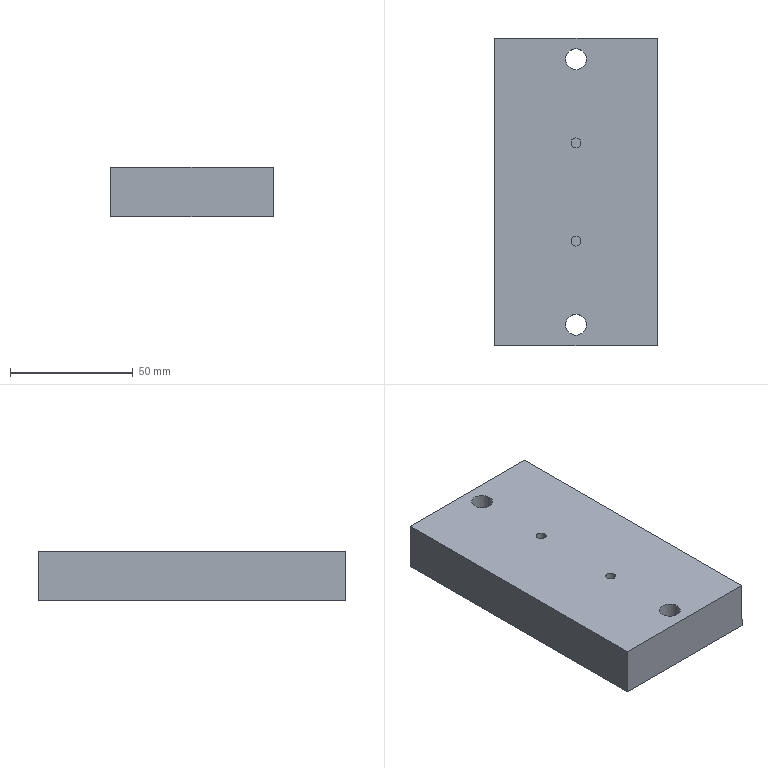NC program | NX | posted with a generic post | part box 65.936 x 125 x 20 mm
Lines 4573 to 6199 of 29196:
(FACE_MILLING_COPY , TOOL : D63)
N9024 T01 M6
N9026 G54
N9028 G17 G0 G90 X86.95 Y-24.269 S4000 M3
N9030 G43 Z37.5 H1
N9032 G94 G1 Z5.033 F5000.
N9034 X77.5 F2000.
N9036 X-77.5
N9038 Y24.269
N9040 X77.5
N9042 X86.95
N9044 G0 Z17.5
N9046 Y-24.269
N9048 G1 Z2.567 F5000.
N9050 X77.5 F2000.
N9052 X-77.5
N9054 Y24.269
N9056 X77.5
N9058 X86.95
N9060 G0 Z17.5
N9062 Y-24.269
N9064 G1 Z0.1 F5000.
N9066 X77.5 F2000.
N9068 X-77.5
N9070 Y24.269
N9072 X77.5
N9074 X86.95
N9076 G0 Z37.5
(FACE_MILLING_COPY_COPY , TOOL : D63)
N9078 Y-24.269
N9080 G1 Z0. F5000.
N9082 X77.5 F1000.
N9084 X-77.5
N9086 Y24.269
N9088 X77.5
N9090 X86.95
N9092 G0 Z37.5
(ZLEVEL_PROFILE_2 , TOOL : D63)
N9094 X86.434 Y-13.072
N9096 Z30.5
N9098 G1 Z-0.462 F5000.
N9100 X45.485 Y-13.396
N9102 X44.426 Y-13.405
N9104 X-45.488
N9106 X-86.438
N9108 G0 Y-15.399 Z-1.423
N9110 G1 X-45.488
N9112 X44.426
N9114 X45.485 Y-15.39
N9116 X86.434 Y-15.066
N9118 G0 Y-17.06 Z-2.385
N9120 G1 X45.485 Y-17.384
N9122 X44.426 Y-17.393
N9124 X-45.488
N9126 X-86.438
N9128 G0 Y-19.386 Z-3.347
N9130 G1 X-45.488
N9132 X44.426
N9134 X45.485 Y-19.378
N9136 X86.434 Y-19.054
N9138 G0 Y-21.048 Z-4.308
N9140 G1 X45.485 Y-21.372
N9142 X44.426 Y-21.38
N9144 X-45.488
N9146 X-86.438
N9148 G0 Y-23.374 Z-5.27
N9150 G1 X-45.488
N9152 X44.426
N9154 X45.485 Y-23.366
N9156 X86.434 Y-23.042
N9158 G0 Y-25.036 Z-6.232
N9160 G1 X45.485 Y-25.36
N9162 X44.426 Y-25.368
N9164 X-45.488
N9166 X-86.438
N9168 G0 Y-27.362 Z-7.193
N9170 G1 X-45.488
N9172 X44.426
N9174 X45.485 Y-27.354
N9176 X86.434 Y-27.029
N9178 G0 Y-29.023 Z-8.155
N9180 G1 X45.485 Y-29.347
N9182 X44.426 Y-29.356
N9184 X-45.488
N9186 X-86.438
N9188 G0 Y-31.35 Z-9.117
N9190 G1 X-45.488
N9192 X44.426
N9194 X45.485 Y-31.341
N9196 X86.434 Y-31.017
N9198 G0 Y-33.011 Z-10.078
N9200 G1 X45.485 Y-33.335
N9202 X44.426 Y-33.344
N9204 X-45.488
N9206 X-86.438
N9208 G0 Y-35.337 Z-11.04
N9210 G1 X-45.488
N9212 X44.426
N9214 X45.485 Y-35.329
N9216 X86.434 Y-35.005
N9218 G0 Y-36.999 Z-12.001
N9220 G1 X45.485 Y-37.323
N9222 X44.426 Y-37.331
N9224 X-45.488
N9226 X-86.438
N9228 G0 Y-39.325 Z-12.963
N9230 G1 X-45.488
N9232 X45.536
N9234 X86.486
N9236 G0 Z30.5
(ZLEVEL_PROFILE_2_COPY , TOOL : D63)
N9238 X-86.435 Y52.145
N9240 G1 Z-0.479
N9242 X-45.485 Y52.148
N9244 X-45.372
N9246 X44.666
N9248 X45.485 Y52.144
N9250 X86.435 Y51.946
N9252 G0 X86.434 Y52.458 Z-1.457
N9254 G1 X45.485 Y52.832
N9256 X45.372 Y52.833
N9258 X-45.372
N9260 X-45.485 Y52.832
N9262 X-86.434 Y52.458
N9264 G0 X-86.435 Y53.316 Z-2.436
N9266 G1 X-45.485 Y53.514
N9268 X-44.666 Y53.518
N9270 X44.666
N9272 X45.485 Y53.514
N9274 X86.435 Y53.316
N9276 G0 X86.434 Y53.829 Z-3.414
N9278 G1 X45.485 Y54.202
N9280 X45.372 Y54.203
N9282 X-45.372
N9284 X-45.485 Y54.202
N9286 X-86.434 Y53.829
N9288 G0 X-86.435 Y54.887 Z-4.393
N9290 G1 X-45.485 Y54.889
N9292 X-45.484
N9294 X44.666
N9296 X45.485 Y54.885
N9298 X86.435 Y54.686
N9300 G0 Y55.372 Z-5.371
N9302 G1 X45.485 Y55.57
N9304 X44.666 Y55.574
N9306 X-44.666
N9308 X-45.485 Y55.57
N9310 X-86.435 Y55.372
N9312 G0 Y56.057 Z-6.35
N9314 G1 X-45.485 Y56.255
N9316 X-44.666 Y56.259
N9318 X44.666
N9320 X45.485 Y56.255
N9322 X86.435 Y56.057
N9324 G0 Y56.742 Z-7.329
N9326 G1 X45.485 Y56.94
N9328 X44.666 Y56.944
N9330 X-44.666
N9332 X-45.485 Y56.94
N9334 X-86.435 Y56.742
N9336 G0 X-86.434 Y57.255 Z-8.307
N9338 G1 X-45.485 Y57.628
N9340 X-45.372 Y57.629
N9342 X45.372
N9344 X45.485 Y57.628
N9346 X86.434 Y57.255
N9348 G0 X86.435 Y58.113 Z-9.286
N9350 G1 X45.485 Y58.311
N9352 X44.666 Y58.315
N9354 X-45.372
N9356 X-45.485 Y58.314
N9358 X-86.434 Y57.94
N9360 G0 Y58.625 Z-10.264
N9362 G1 X-45.485 Y58.999
N9364 X-45.372 Y59.
N9366 X45.372
N9368 X45.485 Y58.999
N9370 X86.434 Y58.625
N9372 G0 X86.435 Y59.483 Z-11.243
N9374 G1 X45.485 Y59.681
N9376 X44.666 Y59.685
N9378 X-44.666
N9380 X-45.485 Y59.681
N9382 X-86.435 Y59.483
N9384 G0 Y60.369 Z-12.221
N9386 G1 X-45.485 Y60.37
N9388 X-45.372
N9390 X44.666
N9392 X45.485 Y60.366
N9394 X86.435 Y60.168
N9396 G0 Y61.055 Z-13.2
N9398 G1 X45.485
N9400 X-45.
N9402 X-45.449 Y61.053
N9404 X-86.398 Y60.798
N9406 G0 Z30.5
(ZLEVEL_PROFILE_2_COPY_COPY , TOOL : D63)
N9408 X-86.435 Y66.087
N9410 Z16.974
N9412 G1 Z-14.388
N9414 X-45.485 Y66.088 F4500.
N9416 X-45.372 Y66.087
N9418 X45.372
N9420 X45.485 Y66.088
N9422 X86.435 Y66.087
N9424 G0 X86.436 Y66.761 Z-15.351
N9426 G1 X45.486 Y66.762
N9428 X45.372
N9430 X-45.372
N9432 X-45.486
N9434 X-86.436 Y66.761
N9436 G0 Y67.435 Z-16.315
N9438 G1 X-45.486 Y67.437
N9440 X-45.372 Y67.436
N9442 X45.372
N9444 X45.486 Y67.437
N9446 X86.436 Y67.435
N9448 G0 Y68.11 Z-17.278
N9450 G1 X45.486 Y68.111
N9452 X45.372
N9454 X-45.372
N9456 X-45.486
N9458 X-86.436 Y68.11
N9460 G0 Y68.784 Z-18.241
N9462 G1 X-45.486 Y68.785
N9464 X-45.485
N9466 X45.485
N9468 X45.486
N9470 X86.436 Y68.784
N9472 G0 Y69.46 Z-19.204
N9474 G1 X45.486
N9476 X-45.486
N9478 X-86.436
N9480 G0 Y70.134 Z-20.168
N9482 G1 X-45.486
N9484 X45.486
N9486 X86.436
N9488 G0 Y70.809 Z-21.131
N9490 G1 X45.486
N9492 X-45.486
N9494 X-86.436
N9496 G0 Y71.483 Z-22.094
N9498 G1 X-45.486 Y71.484
N9500 X-45.372 Y71.483
N9502 X45.372
N9504 X45.486 Y71.484
N9506 X86.436 Y71.483
N9508 G0 Y72.158 Z-23.058
N9510 G1 X45.486
N9512 X45.372
N9514 X-45.372
N9516 X-45.486
N9518 X-86.436
N9520 G0 X-86.435 Y72.832 Z-24.021
N9522 G1 X-45.485 Y72.833
N9524 X-45.372 Y72.832
N9526 X45.372
N9528 X45.485 Y72.833
N9530 X86.435 Y72.832
N9532 G0 Y73.507 Z-24.984
N9534 G1 X45.485
N9536 X-45.485
N9538 X-86.435
N9540 G0 Z16.974
(PLANAR_MILL_1_COPY_COPY_COPY_COPY_1 , TOOL : D63)
N9542 X83.8 Y-66.
N9544 Z9.801
N9546 G1 Y-58.235 Z-19.177 F5000.
N9548 X46. F1200.
N9550 X-46.
N9552 X-83.8
N9554 G0 Y-66. Z9.801
N9556 M5
(PLANAR_MILL_1_COPY_COPY_COPY , TOOL : D6R0)
N9558 T09 M6
N9560 G54
N9562 G17 G0 G90 X-27.791 Y-24.135 S8000 M3
N9564 G43 Z17.075 H9
N9566 G94 G1 Z-12.325 F5000.
N9568 X-39.095 Z-12.404 F2000.
N9570 X-39.333 Y-24.194 Z-12.405
N9572 X-39.547 Y-24.314 Z-12.407
N9574 X-39.721 Y-24.488 Z-12.409
N9576 X-39.841 Y-24.702 Z-12.411
N9578 X-39.9 Y-24.94 Z-12.412
N9580 Y-28.13 Z-12.435
N9582 X-39.841 Y-28.369 Z-12.436
N9584 X-39.721 Y-28.582 Z-12.438
N9586 X-39.547 Y-28.756 Z-12.44
N9588 X-39.333 Y-28.877 Z-12.441
N9590 X-39.095 Y-28.935 Z-12.443
N9592 X39.095 Z-12.989
N9594 X39.333 Y-28.877 Z-12.991
N9596 X39.547 Y-28.756 Z-12.992
N9598 X39.721 Y-28.582 Z-12.994
N9600 X39.841 Y-28.369 Z-12.996
N9602 X39.9 Y-28.13 Z-12.998
N9604 Y-24.94 Z-13.02
N9606 X39.841 Y-24.702 Z-13.022
N9608 X39.721 Y-24.488 Z-13.023
N9610 X39.547 Y-24.314 Z-13.025
N9612 X39.333 Y-24.194 Z-13.027
N9614 X39.095 Y-24.135 Z-13.028
N9616 X-39.095 Z-13.574
N9618 X-39.333 Y-24.194 Z-13.576
N9620 X-39.547 Y-24.314 Z-13.578
N9622 X-39.721 Y-24.488 Z-13.579
N9624 X-39.841 Y-24.702 Z-13.581
N9626 X-39.9 Y-24.94 Z-13.583
N9628 Y-28.13 Z-13.605
N9630 X-39.841 Y-28.369 Z-13.607
N9632 X-39.721 Y-28.582 Z-13.609
N9634 X-39.547 Y-28.756 Z-13.61
N9636 X-39.333 Y-28.877 Z-13.612
N9638 X-39.095 Y-28.935 Z-13.614
N9640 X39.095 Z-14.16
N9642 X39.333 Y-28.877 Z-14.161
N9644 X39.547 Y-28.756 Z-14.163
N9646 X39.721 Y-28.582 Z-14.165
N9648 X39.841 Y-28.369 Z-14.166
N9650 X39.9 Y-28.13 Z-14.168
N9652 Y-24.94 Z-14.19
N9654 X39.841 Y-24.702 Z-14.192
N9656 X39.721 Y-24.488 Z-14.194
N9658 X39.547 Y-24.314 Z-14.196
N9660 X39.333 Y-24.194 Z-14.197
N9662 X39.095 Y-24.135 Z-14.199
N9664 X-39.095 Z-14.745
N9666 X-39.333 Y-24.194 Z-14.747
N9668 X-39.547 Y-24.314 Z-14.748
N9670 X-39.721 Y-24.488 Z-14.75
N9672 X-39.841 Y-24.702 Z-14.752
N9674 X-39.9 Y-24.94 Z-14.753
N9676 Y-28.13 Z-14.776
N9678 X-39.841 Y-28.369 Z-14.777
N9680 X-39.721 Y-28.582 Z-14.779
N9682 X-39.547 Y-28.756 Z-14.781
N9684 X-39.333 Y-28.877 Z-14.783
N9686 X-39.095 Y-28.935 Z-14.784
N9688 X39.095 Z-15.33
N9690 X39.333 Y-28.877 Z-15.332
N9692 X39.547 Y-28.756 Z-15.334
N9694 X39.721 Y-28.582 Z-15.335
N9696 X39.841 Y-28.369 Z-15.337
N9698 X39.9 Y-28.13 Z-15.339
N9700 Y-24.94 Z-15.361
N9702 X39.841 Y-24.702 Z-15.363
N9704 X39.721 Y-24.488 Z-15.364
N9706 X39.547 Y-24.314 Z-15.366
N9708 X39.333 Y-24.194 Z-15.368
N9710 X39.095 Y-24.135 Z-15.37
N9712 X-39.095 Z-15.915
N9714 X-39.333 Y-24.194 Z-15.917
N9716 X-39.547 Y-24.314 Z-15.919
N9718 X-39.721 Y-24.488 Z-15.921
N9720 X-39.841 Y-24.702 Z-15.922
N9722 X-39.9 Y-24.94 Z-15.924
N9724 Y-28.13 Z-15.946
N9726 X-39.841 Y-28.369 Z-15.948
N9728 X-39.721 Y-28.582 Z-15.95
N9730 X-39.547 Y-28.756 Z-15.951
N9732 X-39.333 Y-28.877 Z-15.953
N9734 X-39.095 Y-28.935 Z-15.955
N9736 X39.095 Z-16.501
N9738 X39.333 Y-28.877 Z-16.502
N9740 X39.547 Y-28.756 Z-16.504
N9742 X39.721 Y-28.582 Z-16.506
N9744 X39.841 Y-28.369 Z-16.508
N9746 X39.9 Y-28.13 Z-16.509
N9748 Y-24.94 Z-16.532
N9750 X39.841 Y-24.702 Z-16.533
N9752 X39.721 Y-24.488 Z-16.535
N9754 X39.547 Y-24.314 Z-16.537
N9756 X39.333 Y-24.194 Z-16.538
N9758 X39.095 Y-24.135 Z-16.54
N9760 X-39.095 Z-17.086
N9762 X-39.333 Y-24.194 Z-17.088
N9764 X-39.547 Y-24.314 Z-17.089
N9766 X-39.721 Y-24.488 Z-17.091
N9768 X-39.841 Y-24.702 Z-17.093
N9770 X-39.9 Y-24.94 Z-17.095
N9772 Y-28.13 Z-17.117
N9774 X-39.841 Y-28.369 Z-17.119
N9776 X-39.721 Y-28.582 Z-17.12
N9778 X-39.547 Y-28.756 Z-17.122
N9780 X-39.333 Y-28.877 Z-17.124
N9782 X-39.095 Y-28.935 Z-17.125
N9784 X39.095 Z-17.671
N9786 X39.333 Y-28.877 Z-17.673
N9788 X39.547 Y-28.756 Z-17.675
N9790 X39.721 Y-28.582 Z-17.676
N9792 X39.841 Y-28.369 Z-17.678
N9794 X39.9 Y-28.13 Z-17.68
N9796 Y-24.94 Z-17.702
N9798 X39.841 Y-24.702 Z-17.704
N9800 X39.721 Y-24.488 Z-17.706
N9802 X39.547 Y-24.314 Z-17.707
N9804 X39.333 Y-24.194 Z-17.709
N9806 X39.095 Y-24.135 Z-17.711
N9808 X-39.095 Z-18.257
N9810 X-39.333 Y-24.194 Z-18.258
N9812 X-39.547 Y-24.314 Z-18.26
N9814 X-39.721 Y-24.488 Z-18.262
N9816 X-39.841 Y-24.702 Z-18.263
N9818 X-39.9 Y-24.94 Z-18.265
N9820 Y-28.13 Z-18.287
N9822 X-39.841 Y-28.369 Z-18.289
N9824 X-39.721 Y-28.582 Z-18.291
N9826 X-39.547 Y-28.756 Z-18.293
N9828 X-39.333 Y-28.877 Z-18.294
N9830 X-39.095 Y-28.935 Z-18.296
N9832 X39.095 Z-18.842
N9834 X39.333 Y-28.877 Z-18.844
N9836 X39.547 Y-28.756 Z-18.845
N9838 X39.721 Y-28.582 Z-18.847
N9840 X39.841 Y-28.369 Z-18.849
N9842 X39.9 Y-28.13 Z-18.85
N9844 Y-24.94 Z-18.873
N9846 X39.841 Y-24.702 Z-18.874
N9848 X39.721 Y-24.488 Z-18.876
N9850 X39.547 Y-24.314 Z-18.878
N9852 X39.333 Y-24.194 Z-18.88
N9854 X39.095 Y-24.135 Z-18.881
N9856 X-39.095 Z-19.427
N9858 X-39.333 Y-24.194 Z-19.429
N9860 X-39.547 Y-24.314 Z-19.431
N9862 X-39.721 Y-24.488 Z-19.432
N9864 X-39.841 Y-24.702 Z-19.434
N9866 X-39.9 Y-24.94 Z-19.436
N9868 Y-28.13 Z-19.458
N9870 X-39.841 Y-28.369 Z-19.46
N9872 X-39.721 Y-28.582 Z-19.461
N9874 X-39.547 Y-28.756 Z-19.463
N9876 X-39.333 Y-28.877 Z-19.465
N9878 X-39.095 Y-28.935 Z-19.467
N9880 X39.095 Z-20.012
N9882 X39.333 Y-28.877 Z-20.014
N9884 X39.547 Y-28.756 Z-20.016
N9886 X39.721 Y-28.582 Z-20.018
N9888 X39.841 Y-28.369 Z-20.019
N9890 X39.9 Y-28.13 Z-20.021
N9892 Y-24.94 Z-20.043
N9894 X39.841 Y-24.702 Z-20.045
N9896 X39.721 Y-24.488 Z-20.047
N9898 X39.547 Y-24.314 Z-20.048
N9900 X39.333 Y-24.194 Z-20.05
N9902 X39.095 Y-24.135 Z-20.052
N9904 X0. Z-20.325
N9906 X-39.
N9908 G3 X-39.9 Y-25.035 R0.9
N9910 G1 Y-28.035
N9912 G3 X-39. Y-28.935 R0.9
N9914 G1 X39.
N9916 G3 X39.9 Y-28.035 R0.9
N9918 G1 Y-25.035
N9920 G3 X39. Y-24.135 R0.9
N9922 G1 X0.
N9924 G0 Z17.075
(PLANAR_MILL_1_COPY_COPY_COPY_COPY , TOOL : D6R0)
N9926 X0.75 Y-25.468
N9928 G1 Z-20.275 F5000.
N9930 Z-20.425 F100.
N9932 G41 X1. Y-25.035 D9
N9934 G3 X0. Y-24.035 R1.
N9936 G1 X-39. F800.
N9938 G3 X-40. Y-25.035 R1.
N9940 G1 Y-28.035
N9942 G3 X-39. Y-29.035 R1.
N9944 G1 X39.
N9946 G3 X40. Y-28.035 R1.
N9948 G1 Y-25.035
N9950 G3 X39. Y-24.035 R1.
N9952 G1 X0.
N9954 X-0.3
N9956 G3 X-1.3 Y-25.035 R1.
N9958 G40
N9960 G1 X-1.05 Y-25.468
N9962 Z-20.275
N9964 G0 Z17.075
(CAVITY_MILL , TOOL : D6R0)
N9966 Z30.
N9968 X49.62 Y-37.802
N9970 G1 Z-13.916 F5000.
N9972 X46.02 F4500.
N9974 Y-39.046
N9976 Y-39.219
N9978 Y-41.432
N9980 X46.014 Y-41.446
N9982 X45.8 Y-41.654
N9984 X43.014 Y-44.346
N9986 X43. Y-44.352
N9988 X38.561 Y-44.35
N9990 X38.536 Y-44.346
N9992 X38.533 Y-44.318
N9994 X38.557 Y-44.31
N9996 X38.604 Y-44.3
N9998 X38.723 Y-44.275
N10000 X38.826 Y-44.248
N10002 X38.929 Y-44.218
N10004 X39.066 Y-44.171
N10006 X39.363 Y-44.043
N10008 X39.41 Y-44.019
N10010 X39.754 Y-43.813
N10012 X39.907 Y-43.7
N10014 X40.097 Y-43.536
N10016 X40.276 Y-43.356
N10018 X40.441 Y-43.16
N10020 X40.547 Y-43.012
N10022 X40.75 Y-42.668
N10024 X40.784 Y-42.598
N10026 X40.898 Y-42.325
N10028 X41. Y-41.981
N10030 X41.059 Y-41.638
N10032 X41.08 Y-41.293
N10034 Y-40.953
N10036 Y-40.948
N10038 Y-40.256
N10040 Y-39.144
N10042 X41.2
N10044 G3 X44.3 Y-36.044 R3.1
N10046 G1 Y-35.499
N10048 G3 X46.01 Y-34.155 R3.1
N10050 G1 X46.026 Y-34.157
N10052 X46.02 Y-34.172
N10054 Y-37.802
N10056 X49.62
N10058 G0 Z-13.125
N10060 G1 Z-14.407 F5000.
N10062 X46.02 F4500.
N10064 Y-39.046
N10066 Y-39.219
N10068 Y-41.432
N10070 X46.014 Y-41.446
N10072 X45.8 Y-41.654
N10074 X43.014 Y-44.346
N10076 X43. Y-44.352
N10078 X38.561 Y-44.35
N10080 X38.536 Y-44.346
N10082 X38.533 Y-44.318
N10084 X38.557 Y-44.31
N10086 X38.604 Y-44.3
N10088 X38.723 Y-44.275
N10090 X38.826 Y-44.248
N10092 X38.929 Y-44.218
N10094 X39.066 Y-44.171
N10096 X39.363 Y-44.043
N10098 X39.41 Y-44.019
N10100 X39.754 Y-43.813
N10102 X39.907 Y-43.7
N10104 X40.097 Y-43.536
N10106 X40.276 Y-43.356
N10108 X40.441 Y-43.16
N10110 X40.547 Y-43.012
N10112 X40.75 Y-42.668
N10114 X40.784 Y-42.598
N10116 X40.898 Y-42.325
N10118 X41. Y-41.981
N10120 X41.059 Y-41.638
N10122 X41.08 Y-41.293
N10124 Y-40.953
N10126 Y-40.948
N10128 Y-40.795
N10130 G3 X41.1 Y-40.433 R5.336
N10132 G1 Y-39.144
N10134 X41.2
N10136 G3 X44.3 Y-36.044 R3.1
N10138 G1 Y-35.499
N10140 G3 X46.01 Y-34.155 R3.1
N10142 G1 X46.026 Y-34.157
N10144 X46.02 Y-34.172
N10146 Y-37.802
N10148 X49.62
N10150 G0 Z-13.616
N10152 G1 Z-14.898 F5000.
N10154 X46.02 F4500.
N10156 Y-39.046
N10158 Y-39.219
N10160 Y-41.432
N10162 X46.014 Y-41.446
N10164 X45.8 Y-41.654
N10166 X43.014 Y-44.346
N10168 X43. Y-44.352
N10170 X38.561 Y-44.35
N10172 X38.541 Y-44.352
N10174 Y-44.332
N10176 G3 X41.1 Y-41.21 R3.106
N10178 G1 Y-39.144
N10180 X41.2
N10182 G3 X44.3 Y-36.044 R3.1
N10184 G1 Y-35.499
N10186 G3 X46.01 Y-34.155 R3.1
N10188 G1 X46.026 Y-34.157
N10190 X46.02 Y-34.172
N10192 Y-37.802
N10194 X49.62
N10196 G0 Z-14.107
N10198 G1 Z-15.388 F5000.
N10200 X46.02 F4500.
N10202 Y-39.046
N10204 Y-39.219
N10206 Y-41.432
N10208 X46.014 Y-41.446
N10210 X45.8 Y-41.654
N10212 X43.014 Y-44.346
N10214 X43. Y-44.352
N10216 X38.561 Y-44.35
N10218 X38.541 Y-44.352
N10220 Y-44.332
N10222 G3 X41.1 Y-41.078 R3.12
N10224 G1 Y-39.144
N10226 X41.2
N10228 G3 X44.3 Y-36.044 R3.1
N10230 G1 Y-35.499
N10232 G3 X46.01 Y-34.155 R3.1
N10234 G1 X46.026 Y-34.157
N10236 X46.02 Y-34.172
N10238 Y-37.802
N10240 X49.62
N10242 G0 Z-14.598
N10244 G1 Z-15.879 F5000.
N10246 X46.02 F4500.
N10248 Y-39.046
N10250 Y-39.219
N10252 Y-41.432
N10254 X46.014 Y-41.446
N10256 X45.8 Y-41.654
N10258 X43.014 Y-44.346
N10260 X43. Y-44.352
N10262 X38.561 Y-44.35
N10264 X38.542 Y-44.353
N10266 Y-44.333
N10268 G3 X41.1 Y-41.252 R3.103
N10270 G1 Y-39.144
N10272 X41.2
N10274 G3 X44.3 Y-36.044 R3.1
N10276 G1 Y-35.499
N10278 G3 X46.01 Y-34.155 R3.1
N10280 G1 X46.026 Y-34.157
N10282 X46.02 Y-34.172
N10284 Y-37.802
N10286 X49.62
N10288 G0 Z-15.088
N10290 G1 Z-16.37 F5000.
N10292 X46.02 F4500.
N10294 Y-39.046
N10296 Y-39.219
N10298 Y-41.432
N10300 X46.014 Y-41.446
N10302 X45.8 Y-41.654
N10304 X43.014 Y-44.346
N10306 X43. Y-44.352
N10308 X38.561 Y-44.35
N10310 X38.542 Y-44.353
N10312 X38.541 Y-44.333
N10314 G3 X41.1 Y-41.259 R3.102
N10316 G1 Y-39.144
N10318 X41.2
N10320 G3 X44.3 Y-36.044 R3.1
N10322 G1 Y-35.499
N10324 G3 X46.01 Y-34.155 R3.1
N10326 G1 X46.026 Y-34.157
N10328 X46.02 Y-34.172
N10330 Y-37.802
N10332 X49.62
N10334 G0 Z-15.579
N10336 G1 Z-16.861 F5000.
N10338 X46.02 F4500.
N10340 Y-39.046
N10342 Y-39.219
N10344 Y-41.432
N10346 X46.014 Y-41.446
N10348 X45.8 Y-41.654
N10350 X43.014 Y-44.346
N10352 X43. Y-44.352
N10354 X38.561 Y-44.35
N10356 X38.542 Y-44.353
N10358 X38.541 Y-44.333
N10360 G3 X41.1 Y-41.267 R3.102
N10362 G1 Y-39.144
N10364 X41.2
N10366 G3 X44.3 Y-36.044 R3.1
N10368 G1 Y-35.499
N10370 G3 X46.01 Y-34.155 R3.1
N10372 G1 X46.026 Y-34.157
N10374 X46.02 Y-34.172
N10376 Y-37.802
N10378 X49.62
N10380 G0 Z-16.07
N10382 G1 Z-17.352 F5000.
N10384 X46.02 F4500.
N10386 Y-39.046
N10388 Y-39.219
N10390 Y-41.432
N10392 X46.014 Y-41.446
N10394 X45.8 Y-41.654
N10396 X43.014 Y-44.346
N10398 X43. Y-44.352
N10400 X38.561 Y-44.35
N10402 X38.542 Y-44.353
N10404 X38.541 Y-44.333
N10406 G3 X41.1 Y-41.274 R3.101
N10408 G1 Y-39.144
N10410 X41.2
N10412 G3 X44.3 Y-36.044 R3.1
N10414 G1 Y-35.499
N10416 G3 X46.01 Y-34.155 R3.1
N10418 G1 X46.026 Y-34.157
N10420 X46.02 Y-34.172
N10422 Y-37.802
N10424 X49.62
N10426 G0 Z-16.561
N10428 G1 Z-17.843 F5000.
N10430 X46.02 F4500.
N10432 Y-39.046
N10434 Y-39.219
N10436 Y-41.432
N10438 X46.014 Y-41.446
N10440 X45.8 Y-41.654
N10442 X43.014 Y-44.346
N10444 X43. Y-44.352
N10446 X38.561 Y-44.35
N10448 X38.541 Y-44.352
N10450 Y-44.332
N10452 G3 X41.1 Y-41.282 R3.107
N10454 G1 Y-39.144
N10456 X41.2
N10458 G3 X44.3 Y-36.044 R3.1
N10460 G1 Y-35.499
N10462 G3 X46.01 Y-34.155 R3.1
N10464 G1 X46.026 Y-34.157
N10466 X46.02 Y-34.172
N10468 Y-37.802
N10470 X49.62
N10472 G0 Z-17.052
N10474 G1 Z-18.334 F5000.
N10476 X46.02 F4500.
N10478 Y-39.046
N10480 Y-39.219
N10482 Y-41.432
N10484 X46.014 Y-41.446
N10486 X45.8 Y-41.654
N10488 X43.014 Y-44.346
N10490 X43. Y-44.352
N10492 X38.561 Y-44.35
N10494 X38.542 Y-44.353
N10496 Y-44.334
N10498 G3 X41.1 Y-41.289 R3.096
N10500 G1 Y-39.144
N10502 X41.2
N10504 G3 X44.3 Y-36.044 R3.1
N10506 G1 Y-35.499
N10508 G3 X46.01 Y-34.155 R3.1
N10510 G1 X46.026 Y-34.157
N10512 X46.02 Y-34.172
N10514 Y-37.802
N10516 X49.62
N10518 G0 Z-17.543
N10520 G1 Z-18.825 F5000.
N10522 X46.02 F4500.
N10524 Y-39.046
N10526 Y-39.219
N10528 Y-41.432
N10530 X46.014 Y-41.446
N10532 X45.8 Y-41.654
N10534 X43.014 Y-44.346
N10536 X43. Y-44.352
N10538 X38.561 Y-44.35
N10540 X38.543 Y-44.354
N10542 X38.542 Y-44.335
N10544 G3 X41.049 Y-41.827 R3.079
N10546 X41.1 Y-40.948 R3.891
N10548 G1 Y-39.144
N10550 X41.2
N10552 G3 X44.3 Y-36.044 R3.1
N10554 G1 Y-35.499
N10556 G3 X46.01 Y-34.155 R3.1
N10558 G1 X46.026 Y-34.157
N10560 X46.02 Y-34.172
N10562 Y-37.802
N10564 X49.62
N10566 G0 Z-18.034
N10568 X47.015 Y-45.486
N10570 G1 Z-19.202 F5000.
N10572 X44.514 Y-42.897 F4500.
N10574 X43.014 Y-44.346
N10576 X43. Y-44.352
N10578 X38.561 Y-44.35
N10580 X38.542 Y-44.353
N10582 X38.541 Y-44.333
N10584 G3 X41.029 Y-41.939 R3.1
N10586 X41.1 Y-40.948 R4.04
N10588 G1 Y-40.466
N10590 X46.
N10592 X46.02
N10594 Y-41.432
N10596 X46.014 Y-41.446
N10598 X45.8 Y-41.654
N10600 X44.514 Y-42.897
N10602 X47.015 Y-45.486
N10604 G0 Z-18.525
N10606 G1 Z-19.58 F5000.
N10608 X44.514 Y-42.897 F4500.
N10610 X43.014 Y-44.346
N10612 X43. Y-44.352
N10614 X38.561 Y-44.35
N10616 X38.541 Y-44.352
N10618 Y-44.332
N10620 G3 X41.043 Y-41.875 R3.097
N10622 G1 X45.544
N10624 X45.572
N10626 X45.562 Y-41.884
N10628 X44.514 Y-42.897
N10630 X47.015 Y-45.486
N10632 G0 Z-18.902
N10634 X40.779 Y-47.951
N10636 G1 Z-19.957 F5000.
N10638 X40.78 Y-44.351 F4500.
N10640 X38.561 Y-44.35
N10642 X38.542 Y-44.353
N10644 X38.541 Y-44.333
N10646 G3 X40.366 Y-43.284 R3.103
N10648 G1 X44.085
N10650 X44.115 Y-43.282
N10652 X44.104 Y-43.293
N10654 X43.014 Y-44.346
N10656 X43. Y-44.352
N10658 X40.78 Y-44.351
N10660 X40.779 Y-47.951
N10662 G0 Z30.
N10664 X0. Y-28.415
N10666 G1 Z-13.916 F5000.
N10668 Y-32.015 F4500.
N10670 X35.9
N10672 Y-32.035
N10674 Y-35.789
N10676 X35.616
N10678 X-35.9
N10680 Y-32.035
N10682 Y-32.015
N10684 X0.
N10686 Y-28.415
N10688 G0 Z-13.125
N10690 G1 Z-14.407 F5000.
N10692 Y-32.015 F4500.
N10694 X35.9
N10696 Y-32.035
N10698 Y-35.65
N10700 X-35.9
N10702 Y-32.035
N10704 Y-32.015
N10706 X0.
N10708 Y-28.415
N10710 G0 Z-13.616
N10712 G1 Z-14.898 F5000.
N10714 Y-32.015 F4500.
N10716 X35.9
N10718 Y-32.035
N10720 Y-35.518
N10722 X-35.9
N10724 Y-32.035
N10726 Y-32.015
N10728 X0.
N10730 Y-28.415
N10732 G0 Z-14.107
N10734 G1 Z-15.388 F5000.
N10736 Y-32.015 F4500.
N10738 X35.9
N10740 Y-32.035
N10742 Y-35.387
N10744 X-35.9
N10746 Y-32.035
N10748 Y-32.015
N10750 X0.
N10752 Y-28.415
N10754 G0 Z-14.598
N10756 G1 Z-15.879 F5000.
N10758 Y-32.015 F4500.
N10760 X35.9
N10762 Y-32.035
N10764 Y-35.255
N10766 X35.61
N10768 X35.27 Y-35.274
N10770 G2 X34.859 Y-35.289 R1.231
N10772 G3 X34.39 Y-35.255 R3.884
N10774 G1 X0.61
N10776 G3 X0. Y-35.313 R3.285
N10778 X-0.61 Y-35.255 R3.616
N10780 G1 X-34.39
N10782 G3 X-34.862 Y-35.289 R3.884
N10784 G2 X-35.27 Y-35.273 R1.193
N10786 G1 X-35.61 Y-35.255
N10788 X-35.9
N10790 Y-32.035
N10792 Y-32.015
N10794 X0.
N10796 Y-28.415
N10798 G0 Z-15.088
N10800 G1 Z-16.37 F5000.
N10802 Y-32.015 F4500.
N10804 X35.9
N10806 Y-32.035
N10808 Y-35.124
N10810 X35.8
N10812 G3 X34.998 Y-35.226 R2.948
N10814 X34.231 Y-35.124 R3.08
N10816 G1 X34.2
N10818 X0.8
N10820 G3 X0. Y-35.226 R3.067
N10822 X-0.8 Y-35.124 R3.164
N10824 G1 X-34.2
N10826 G3 X-35.002 Y-35.227 R3.207
N10828 X-35.8 Y-35.124 R2.985
N10830 G1 X-35.9
N10832 Y-32.035
N10834 Y-32.015
N10836 X0.
N10838 Y-28.415
N10840 G0 Z-15.579
N10842 G1 Z-16.861 F5000.
N10844 Y-32.015 F4500.
N10846 X35.9
N10848 Y-32.035
N10850 Y-34.992
N10852 X35.618
N10854 G3 X35.169 Y-35.024 R3.541
N10856 G2 X34.578 Y-34.999 R1.703
N10858 G1 X34.382 Y-34.992
N10860 X0.618
N10862 G3 X0. Y-35.052 R3.363
N10864 X-0.618 Y-34.992 R3.433
N10866 G1 X-34.382
N10868 G3 X-34.853 Y-35.028 R3.234
N10870 G2 X-35.27 Y-35.011 R1.114
N10872 G1 X-35.618 Y-34.992
N10874 X-35.9
N10876 Y-32.035
N10878 Y-32.015
N10880 X0.
N10882 Y-28.415
N10884 G0 Z-16.07
N10886 G1 Z-17.352 F5000.
N10888 Y-32.015 F4500.
N10890 X35.9
N10892 Y-32.035
N10894 Y-34.861
N10896 X-35.9
N10898 Y-32.035
N10900 Y-32.015
N10902 X0.
N10904 Y-28.415
N10906 G0 Z-16.561
N10908 G1 Z-17.843 F5000.
N10910 Y-32.015 F4500.
N10912 X35.9
N10914 Y-32.035
N10916 Y-34.729
N10918 X-35.9
N10920 Y-32.035
N10922 Y-32.015
N10924 X0.
N10926 Y-28.415
N10928 G0 Z-17.052
N10930 G1 Z-18.334 F5000.
N10932 Y-32.015 F4500.
N10934 X35.9
N10936 Y-32.035
N10938 Y-34.598
N10940 X-35.9
N10942 Y-32.035
N10944 Y-32.015
N10946 X0.
N10948 Y-28.415
N10950 G0 Z-17.543
N10952 G1 Z-18.825 F5000.
N10954 Y-32.015 F4500.
N10956 X35.9
N10958 Y-32.035
N10960 Y-34.467
N10962 X-35.9
N10964 Y-32.035
N10966 Y-32.015
N10968 X0.
N10970 Y-28.415
N10972 G0 Z30.
N10974 X-49.62 Y-37.806
N10976 G1 Z-13.916 F5000.
N10978 X-46.02 F4500.
N10980 Y-34.376
N10982 Y-34.375
N10984 X-46.01 Y-34.181
N10986 X-46.003 Y-34.167
N10988 G3 X-44.3 Y-35.499 R3.1
N10990 G1 Y-36.044
N10992 G3 X-41.2 Y-39.144 R3.1
N10994 G1 X-41.08
N10996 X-41.07 Y-40.256
N10998 Y-40.433
N11000 Y-40.948
N11002 Y-41.294
N11004 X-41.059 Y-41.638
N11006 X-41. Y-41.981
N11008 X-40.898 Y-42.325
N11010 X-40.784 Y-42.598
N11012 X-40.75 Y-42.668
N11014 X-40.547 Y-43.012
N11016 X-40.441 Y-43.16
N11018 X-40.276 Y-43.356
N11020 X-40.097 Y-43.536
N11022 X-39.907 Y-43.7
N11024 X-39.754 Y-43.813
N11026 X-39.41 Y-44.019
N11028 X-39.363 Y-44.043
N11030 X-39.066 Y-44.171
N11032 X-38.929 Y-44.218
N11034 X-38.826 Y-44.248
N11036 X-38.723 Y-44.275
N11038 X-38.547 Y-44.312
N11040 X-38.523 Y-44.321
N11042 X-38.526 Y-44.349
N11044 X-38.551 Y-44.352
N11046 X-42.956
N11048 X-42.968 Y-44.347
N11050 X-42.995 Y-44.326
N11052 X-43.235 Y-44.13
N11054 X-43.237 Y-44.129
N11056 X-45.442 Y-42.
N11058 X-46.014 Y-41.446
N11060 X-46.02 Y-41.432
N11062 Y-39.219
N11064 Y-39.046
N11066 Y-37.806
N11068 X-49.62
N11070 G0 Z-13.125
N11072 G1 Z-14.407 F5000.
N11074 X-46.02 F4500.
N11076 Y-34.376
N11078 Y-34.375
N11080 X-46.01 Y-34.181
N11082 X-46.003 Y-34.167
N11084 G3 X-44.3 Y-35.499 R3.1
N11086 G1 Y-36.044
N11088 G3 X-41.2 Y-39.144 R3.1
N11090 G1 X-41.1
N11092 Y-40.433
N11094 G3 X-41.07 Y-40.941 R3.966
N11096 G1 Y-40.948
N11098 Y-41.294
N11100 X-41.059 Y-41.638
N11102 X-41. Y-41.981
N11104 X-40.898 Y-42.325
N11106 X-40.784 Y-42.598
N11108 X-40.75 Y-42.668
N11110 X-40.547 Y-43.012
N11112 X-40.441 Y-43.16
N11114 X-40.276 Y-43.356
N11116 X-40.097 Y-43.536
N11118 X-39.907 Y-43.7
N11120 X-39.754 Y-43.813
N11122 X-39.41 Y-44.019
N11124 X-39.363 Y-44.043
N11126 X-39.066 Y-44.171
N11128 X-38.929 Y-44.218
N11130 X-38.826 Y-44.248
N11132 X-38.723 Y-44.275
N11134 X-38.547 Y-44.312
N11136 X-38.523 Y-44.321
N11138 X-38.526 Y-44.349
N11140 X-38.551 Y-44.352
N11142 X-42.956
N11144 X-42.968 Y-44.347
N11146 X-42.995 Y-44.326
N11148 X-43.235 Y-44.13
N11150 X-43.237 Y-44.129
N11152 X-45.442 Y-42.
N11154 X-46.014 Y-41.446
N11156 X-46.02 Y-41.432
N11158 Y-39.219
N11160 Y-39.046
N11162 Y-37.806
N11164 X-49.62
N11166 G0 Z-13.616
N11168 G1 Z-14.898 F5000.
N11170 X-46.02 F4500.
N11172 Y-34.376
N11174 Y-34.375
N11176 X-46.01 Y-34.181
N11178 X-46.003 Y-34.167
N11180 G3 X-44.3 Y-35.499 R3.1
N11182 G1 Y-36.044
N11184 G3 X-41.2 Y-39.144 R3.1
N11186 G1 X-41.1
N11188 Y-41.21
N11190 G3 X-38.531 Y-44.334 R3.108
N11192 G1 Y-44.354
N11194 X-38.551 Y-44.352
N11196 X-42.956
N11198 X-42.968 Y-44.347
N11200 X-42.995 Y-44.326
N11202 X-43.235 Y-44.13
N11204 X-43.237 Y-44.129
N11206 X-45.442 Y-42.
N11208 X-46.014 Y-41.446
N11210 X-46.02 Y-41.432
N11212 Y-39.219
N11214 Y-39.046
N11216 Y-37.806
N11218 X-49.62
N11220 G0 Z-14.107
N11222 G1 Z-15.388 F5000.
N11224 X-46.02 F4500.
N11226 Y-34.376
N11228 Y-34.375
N11230 X-46.01 Y-34.181
N11232 X-46.003 Y-34.167
N11234 G3 X-44.3 Y-35.499 R3.1
N11236 G1 Y-36.044
N11238 G3 X-41.2 Y-39.144 R3.1
N11240 G1 X-41.1
N11242 Y-41.078
N11244 X-41.099 Y-41.292
N11246 G3 X-38.531 Y-44.334 R3.104
N11248 G1 Y-44.354
N11250 X-38.551 Y-44.352
N11252 X-42.956
N11254 X-42.968 Y-44.347
N11256 X-42.995 Y-44.326
N11258 X-43.235 Y-44.13
N11260 X-43.237 Y-44.129
N11262 X-45.442 Y-42.
N11264 X-46.014 Y-41.446
N11266 X-46.02 Y-41.432
N11268 Y-39.219
N11270 Y-39.046
N11272 Y-37.806
N11274 X-49.62
N11276 G0 Z-14.598
N11278 G1 Z-15.879 F5000.
N11280 X-46.02 F4500.
N11282 Y-34.376
N11284 Y-34.375
N11286 X-46.01 Y-34.181
N11288 X-46.003 Y-34.167
N11290 G3 X-44.3 Y-35.499 R3.1
N11292 G1 Y-36.044
N11294 G3 X-41.2 Y-39.144 R3.1
N11296 G1 X-41.1
N11298 Y-41.259
N11300 G3 X-38.531 Y-44.335 R3.105
N11302 G1 Y-44.355
N11304 X-38.551 Y-44.352
N11306 X-42.956
N11308 X-42.968 Y-44.347
N11310 X-42.995 Y-44.326
N11312 X-43.235 Y-44.13
N11314 X-43.237 Y-44.129
N11316 X-45.442 Y-42.
N11318 X-46.014 Y-41.446
N11320 X-46.02 Y-41.432
N11322 Y-39.219
N11324 Y-39.046
N11326 Y-37.806
N11328 X-49.62
N11330 G0 Z-15.088
N11332 G1 Z-16.37 F5000.
N11334 X-46.02 F4500.
N11336 Y-34.376
N11338 Y-34.375
N11340 X-46.01 Y-34.181
N11342 X-46.003 Y-34.167
N11344 G3 X-44.3 Y-35.499 R3.1
N11346 G1 Y-36.044
N11348 G3 X-41.2 Y-39.144 R3.1
N11350 G1 X-41.1
N11352 Y-41.268
N11354 G3 X-38.531 Y-44.335 R3.104
N11356 G1 Y-44.355
N11358 X-38.551 Y-44.352
N11360 X-42.956
N11362 X-42.968 Y-44.347
N11364 X-42.995 Y-44.326
N11366 X-43.235 Y-44.13
N11368 X-43.237 Y-44.129
N11370 X-45.442 Y-42.
N11372 X-46.014 Y-41.446
N11374 X-46.02 Y-41.432
N11376 Y-39.219
N11378 Y-39.046
N11380 Y-37.806
N11382 X-49.62
N11384 G0 Z-15.579
N11386 G1 Z-16.861 F5000.
N11388 X-46.02 F4500.
N11390 Y-34.376
N11392 Y-34.375
N11394 X-46.01 Y-34.181
N11396 X-46.003 Y-34.167
N11398 G3 X-44.3 Y-35.499 R3.1
N11400 G1 Y-36.044
N11402 G3 X-41.2 Y-39.144 R3.1
N11404 G1 X-41.1
N11406 Y-41.276
N11408 G3 X-38.531 Y-44.335 R3.103
N11410 G1 Y-44.355
N11412 X-38.551 Y-44.352
N11414 X-42.956
N11416 X-42.968 Y-44.347
N11418 X-42.995 Y-44.326
N11420 X-43.235 Y-44.13
N11422 X-43.237 Y-44.129
N11424 X-45.442 Y-42.
N11426 X-46.014 Y-41.446
N11428 X-46.02 Y-41.432
N11430 Y-39.219
N11432 Y-39.046
N11434 Y-37.806
N11436 X-49.62
N11438 G0 Z-16.07
N11440 G1 Z-17.352 F5000.
N11442 X-46.02 F4500.
N11444 Y-34.376
N11446 Y-34.375
N11448 X-46.01 Y-34.181
N11450 X-46.003 Y-34.167
N11452 G3 X-44.3 Y-35.499 R3.1
N11454 G1 Y-36.044
N11456 G3 X-41.2 Y-39.144 R3.1
N11458 G1 X-41.1
N11460 Y-41.284
N11462 G3 X-38.531 Y-44.335 R3.102
N11464 G1 Y-44.354
N11466 X-38.551 Y-44.352
N11468 X-42.956
N11470 X-42.968 Y-44.347
N11472 X-42.995 Y-44.326
N11474 X-43.235 Y-44.13
N11476 X-43.237 Y-44.129
N11478 X-45.442 Y-42.
N11480 X-46.014 Y-41.446
N11482 X-46.02 Y-41.432
N11484 Y-39.219
N11486 Y-39.046
N11488 Y-37.806
N11490 X-49.62
N11492 G0 Z-16.561
N11494 G1 Z-17.843 F5000.
N11496 X-46.02 F4500.
N11498 Y-34.376
N11500 Y-34.375
N11502 X-46.01 Y-34.181
N11504 X-46.003 Y-34.167
N11506 G3 X-44.3 Y-35.499 R3.1
N11508 G1 Y-36.044
N11510 G3 X-41.2 Y-39.144 R3.1
N11512 G1 X-41.1
N11514 Y-41.292
N11516 G3 X-38.531 Y-44.335 R3.102
N11518 G1 Y-44.354
N11520 X-38.551 Y-44.352
N11522 X-42.956
N11524 X-42.968 Y-44.347
N11526 X-42.995 Y-44.326
N11528 X-43.235 Y-44.13
N11530 X-43.237 Y-44.129
N11532 X-45.442 Y-42.
N11534 X-46.014 Y-41.446
N11536 X-46.02 Y-41.432
N11538 Y-39.219
N11540 Y-39.046
N11542 Y-37.806
N11544 X-49.62
N11546 G0 Z-17.052
N11548 G1 Z-18.334 F5000.
N11550 X-46.02 F4500.
N11552 Y-34.376
N11554 Y-34.375
N11556 X-46.01 Y-34.181
N11558 X-46.003 Y-34.167
N11560 G3 X-44.3 Y-35.499 R3.1
N11562 G1 Y-36.044
N11564 G3 X-41.2 Y-39.144 R3.1
N11566 G1 X-41.1
N11568 Y-40.948
N11570 G3 X-41.091 Y-41.486 R5.566
N11572 X-38.531 Y-44.335 R3.096
N11574 G1 Y-44.355
N11576 X-38.551 Y-44.352
N11578 X-42.956
N11580 X-42.968 Y-44.347
N11582 X-42.995 Y-44.326
N11584 X-43.235 Y-44.13
N11586 X-43.237 Y-44.129
N11588 X-45.442 Y-42.
N11590 X-46.014 Y-41.446
N11592 X-46.02 Y-41.432
N11594 Y-39.219
N11596 Y-39.046
N11598 Y-37.806
N11600 X-49.62
N11602 G0 Z-17.543
N11604 G1 Z-18.825 F5000.
N11606 X-46.02 F4500.
N11608 Y-34.376
N11610 Y-34.375
N11612 X-46.01 Y-34.181
N11614 X-46.003 Y-34.167
N11616 G3 X-44.3 Y-35.499 R3.1
N11618 G1 Y-36.044
N11620 G3 X-41.2 Y-39.144 R3.1
N11622 G1 X-41.1
N11624 Y-40.948
N11626 G3 X-41.079 Y-41.64 R4.037
N11628 X-38.531 Y-44.335 R3.1
N11630 G1 Y-44.355
N11632 X-38.551 Y-44.352
N11634 X-42.956
N11636 X-42.968 Y-44.347
N11638 X-42.995 Y-44.326
N11640 X-43.235 Y-44.13
N11642 X-43.237 Y-44.129
N11644 X-45.442 Y-42.
N11646 X-46.014 Y-41.446
N11648 X-46.02 Y-41.432
N11650 Y-39.219
N11652 Y-39.046
N11654 Y-37.806
N11656 X-49.62
N11658 G0 Z-18.034
N11660 X-47.001 Y-45.499
N11662 G1 Z-19.202 F5000.
N11664 X-44.501 Y-42.908 F4500.
N11666 X-45.442 Y-42.
N11668 X-46.014 Y-41.446
N11670 X-46.02 Y-41.432
N11672 Y-40.466
N11674 X-46.
N11676 X-41.1
N11678 Y-40.948
N11680 G3 X-41.079 Y-41.64 R4.025
N11682 X-38.531 Y-44.335 R3.1
N11684 G1 Y-44.355
N11686 X-38.551 Y-44.352
N11688 X-42.956
N11690 X-42.968 Y-44.347
N11692 X-42.995 Y-44.326
N11694 X-43.235 Y-44.13
N11696 X-43.237 Y-44.129
N11698 X-44.501 Y-42.908
N11700 X-47.001 Y-45.499
N11702 G0 Z-18.525
N11704 G1 Z-19.58 F5000.
N11706 X-44.501 Y-42.908 F4500.
N11708 X-45.442 Y-42.
N11710 X-45.562 Y-41.884
N11712 X-45.572 Y-41.874
N11714 X-45.544 Y-41.875
N11716 X-41.045
N11718 G3 X-38.728 Y-44.294 R3.108
N11720 X-38.531 Y-44.335 R3.068
N11722 G1 Y-44.355
N11724 X-38.551 Y-44.352
N11726 X-42.956
N11728 X-42.968 Y-44.347
N11730 X-42.995 Y-44.326
N11732 X-43.235 Y-44.13
N11734 X-43.237 Y-44.129
N11736 X-44.501 Y-42.908
N11738 X-47.001 Y-45.499
N11740 G0 Z-18.902
N11742 X-40.753 Y-47.952
N11744 G1 Z-19.957 F5000.
N11746 Y-44.352 F4500.
N11748 X-42.956
N11750 X-42.968 Y-44.347
N11752 X-42.995 Y-44.326
N11754 X-43.235 Y-44.13
N11756 X-43.237 Y-44.129
N11758 X-44.103 Y-43.293
N11760 X-44.114 Y-43.282
N11762 X-44.085 Y-43.284
N11764 X-40.369
N11766 G3 X-38.728 Y-44.294 R3.127
N11768 X-38.531 Y-44.335 R3.057
N11770 G1 Y-44.355
N11772 X-38.551 Y-44.352
N11774 X-40.753
N11776 Y-47.952
N11778 G0 Z30.
(PLANAR_PROFILE , TOOL : D6R0)
N11780 X49.9 Y-52.04
N11782 Z13.542
N11784 G1 Y-44.016 Z-16.402 F5000.
N11786 X46. F3000.
N11788 X-46.
N11790 X-49.9
N11792 G0 Y-43.757 Z-17.368
N11794 G1 X-46.
N11796 X46.
N11798 X49.9
N11800 G0 Y-43.499 Z-18.334
N11802 G1 X46.
N11804 X-46.
N11806 X-49.9
N11808 G0 Y-43.24 Z-19.3
N11810 G1 X-46.
N11812 X46.
N11814 X49.9
N11816 G0 Y-42.981 Z-20.266
N11818 G1 X46.
N11820 X-46.
N11822 X-49.9
N11824 G0 Y-42.877 Z-20.652
N11826 G1 X-46.
N11828 X46.
N11830 X49.9
N11832 G0 Y-52.04 Z13.542
(CAVITY_MILL_COPY_1 , TOOL : D6R0)
N11834 G19 Y8.968 Z-1.212
N11836 X-76.
N11838 G1 X-45.1 F5000.
N11840 Y10.531 Z-4.454 F2000.
N11842 Y-8.027 Z-13.405
N11844 Y-31.035
N11846 Y-31.042 Z-13.404
N11848 Y-31.055 Z-13.425
N11850 Z-15.794
N11852 Y-35.631
N11854 Y-35.641 Z-15.797
N11856 Y-35.65 Z-15.794
N11858 Y-35.833
N11860 Y-35.836
N11862 Y-35.922 Z-15.804
N11864 Y-35.942 Z-15.818
N11866 Y-35.94 Z-15.825
N11868 Y34.571
N11870 G2 Y40.387 Z-18.852 R7.1
N11872 G1 Y43.379 Z-23.125
N11874 Y43.38 Z-23.124
N11876 Y43.395 Z-23.104
N11878 Y43.384 Z-23.097
N11880 Y40.441 Z-18.894
N11882 G3 Y35.118 Z-15.796 R7.147
N11884 G1 Y33.429 Z-13.413
N11886 Y33.431 Z-13.402
N11888 Y33.413 Z-13.405
N11890 Y29.223
N11892 Y19.829 Z0.011
N11894 Y19.825 Z0.026
N11896 Y19.804 Z0.018
N11898 Y10.531 Z-4.454
N11900 Y12.486 Z-8.507
N11902 Y6.645 Z-11.325
N11904 Y2.536 Z-12.264
N11906 Y6.645 Z-11.325
N11908 Y22.273
N11910 Y25.007 Z-12.748
N11912 Y22.273 Z-11.325
N11914 Y18.328 Z-5.69
N11916 Y12.486 Z-8.507
N11918 Y10.922 Z-5.265
N11920 G0 X-76.
(CAVITY_MILL_COPY_1_COPY_1 , TOOL : D6R0)
N11922 Y8.864 Z-1.262
N11924 G1 X-45. F5000.
N11926 Y10.428 Z-4.504 F1200.
N11928 Y-8.027 Z-13.405
N11930 Y-31.035
N11932 Y-31.056 Z-13.418
N11934 Y-31.055 Z-13.425
N11936 Z-15.903
N11938 Y-36.026 Z-15.904
N11940 Y-36.047 Z-15.917
N11942 Y-36.046 Z-15.924
N11944 Y-36.044 Z-15.925
N11946 Y34.571
N11948 G2 Y40.305 Z-18.91 R7.
N11950 G1 Y43.354 Z-23.263
N11952 Y43.359 Z-23.27
N11954 Y43.374 Z-23.25
N11956 Y43.364 Z-23.242
N11958 Y40.529 Z-19.194
N11960 Y40.215 Z-18.745
N11962 G3 Y35.589 Z-15.973 R7.019
N11964 G1 Y35.584
N11966 Y35.567 Z-15.975
N11968 Y35.341 Z-15.947
N11970 Y35.194 Z-15.9
N11972 Y33.429 Z-13.413
N11974 Y33.431 Z-13.402
N11976 Y33.413 Z-13.405
N11978 Y29.223
N11980 Y19.829 Z0.011
N11982 Y19.825 Z0.026
N11984 Y19.804 Z0.018
N11986 Y10.428 Z-4.504
N11988 Y12.383 Z-8.557
N11990 Y6.437 Z-11.425
N11992 Y2.328 Z-12.364
N11994 Y6.437 Z-11.425
N11996 Y22.343
N11998 Y25.077 Z-12.848
N12000 Y22.343 Z-11.425
N12002 Y18.328 Z-5.69
N12004 Y12.383 Z-8.557
N12006 Y10.819 Z-5.315
N12008 G0 X-76.
(CAVITY_MILL_COPY_1_COPY_2 , TOOL : D6R0)
N12010 X76.
N12012 Y8.968 Z-1.212
N12014 G1 X45.1 F5000.
N12016 Y10.531 Z-4.454 F2000.
N12018 Y19.804 Z0.018
N12020 Y19.81 Z0.026
N12022 Y19.829 Z0.011
N12024 Y29.223 Z-13.405
N12026 Y33.413
N12028 Z-13.402
N12030 Y33.429 Z-13.413
N12032 Y35.118 Z-15.796
N12034 G2 Y40.484 Z-18.956 R7.177
N12036 G1 Y43.443 Z-23.181
N12038 Y43.453 Z-23.203
N12040 Y43.438 Z-23.208
N12042 Y43.436 Z-23.206
N12044 Y40.387 Z-18.852
N12046 G3 Y34.571 Z-15.825 R7.1
N12048 G1 Y-36.044
N12050 Y-36.05
N12052 Z-15.815
N12054 Y-36.051 Z-15.794
N12056 Y-36.03 Z-15.795
N12058 Y-35.646
N12060 Y-34.136
N12062 Y-34.133
N12064 Y-34.131
N12066 Y-31.055
N12068 Z-13.425
N12070 Y-31.056 Z-13.404
N12072 Y-31.035 Z-13.405
N12074 Y-8.027
N12076 Y10.531 Z-4.454
N12078 Y12.486 Z-8.507
N12080 Y18.328 Z-5.69
N12082 Y22.273 Z-11.325
N12084 Y25.007 Z-12.748
N12086 Y22.273 Z-11.325
N12088 Y6.645
N12090 Y2.536 Z-12.264
N12092 Y6.645 Z-11.325
N12094 Y12.486 Z-8.507
N12096 Y10.922 Z-5.265
N12098 G0 X76.
(CAVITY_MILL_COPY_1_COPY_2_COPY , TOOL : D6R0)
N12100 Y8.864 Z-1.262
N12102 G1 X45. F5000.
N12104 Y10.428 Z-4.504 F1200.
N12106 Y19.804 Z0.018
N12108 Y19.81 Z0.026
N12110 Y19.829 Z0.011
N12112 Y29.223 Z-13.405
N12114 Y33.413
N12116 Z-13.402
N12118 Y33.429 Z-13.413
N12120 Y35.194 Z-15.9
N12122 Y35.341 Z-15.939
N12124 Y35.571 Z-15.966
N12126 Y35.572
N12128 Y35.591 Z-15.969
N12130 G2 Y40.139 Z-18.627 R7.023
N12132 G1 Y40.225 Z-18.744
N12134 Y40.572 Z-19.24
N12136 Y43.372 Z-23.239
N12138 Y43.382 Z-23.261
N12140 Y43.367 Z-23.267
N12142 Y43.36 Z-23.272
N12144 Y43.354 Z-23.263
N12146 Y40.305 Z-18.91
N12148 G3 Y34.571 Z-15.925 R7.
N12150 G1 Y-36.044
N12152 Y-36.045 Z-15.916
N12154 Y-36.046 Z-15.895
N12156 Y-36.025 Z-15.896
N12158 Y-31.055
N12160 Z-13.425
N12162 Y-31.056 Z-13.404
N12164 Y-31.035 Z-13.405
N12166 Y-8.027
N12168 Y10.428 Z-4.504
N12170 Y12.383 Z-8.557
N12172 Y18.328 Z-5.69
N12174 Y22.343 Z-11.425
N12176 Y25.077 Z-12.848
N12178 Y22.343 Z-11.425
N12180 Y6.437
N12182 Y2.328 Z-12.364
N12184 Y6.437 Z-11.425
N12186 Y12.383 Z-8.557
N12188 Y10.819 Z-5.315
N12190 G0 X76.
N12192 M5